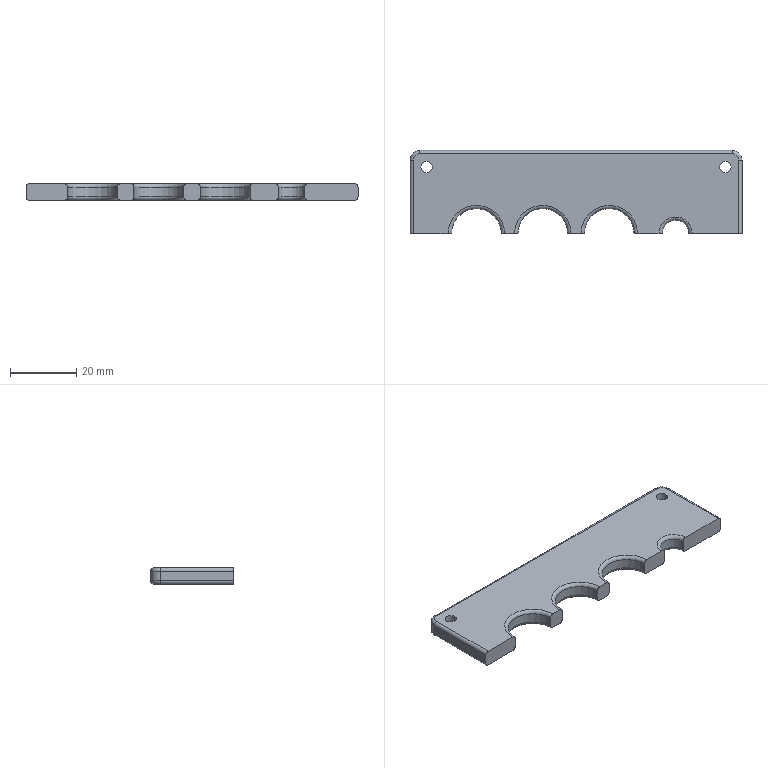Part | SolidWorks | features Fillet 2, Extrusion 1, HoleWzd 1, ICE 1 | 1 solid | 42 faces | box 100 x 25 x 5 mm | volume 10800 mm3 | cylinder 16 | torus 12 | plane 10 | cone 4 | commonest cylinder face diameters 2 x6 3.4 x4 15 x3 6 x2 8 x1
STEP:
#1=CARTESIAN_POINT('',(6.7,20.,1.66));
#2=VERTEX_POINT('',#1);
#3=CARTESIAN_POINT('',(3.3,20.,1.66));
#4=VERTEX_POINT('',#3);
#5=CARTESIAN_POINT('',(5.,20.,1.66));
#6=DIRECTION('',(0.,0.,-1.));
#7=DIRECTION('',(-1.,0.,0.));
#8=AXIS2_PLACEMENT_3D('',#5,#6,#7);
#9=CIRCLE('',#8,1.7);
#10=EDGE_CURVE('',#2,#4,#9,.T.);
#11=ORIENTED_EDGE('',*,*,#10,.F.);
#12=CARTESIAN_POINT('',(8.36,20.,0.));
#13=VERTEX_POINT('',#12);
#14=CARTESIAN_POINT('',(8.36,20.,0.));
#15=DIRECTION('',(0.7071,0.,-0.7071));
#16=VECTOR('',#15,1000.);
#17=LINE('',#14,#16);
#18=EDGE_CURVE('',#2,#13,#17,.T.);
#19=ORIENTED_EDGE('',*,*,#18,.T.);
#20=CARTESIAN_POINT('',(1.64,20.,0.));
#21=VERTEX_POINT('',#20);
#22=CARTESIAN_POINT('',(5.,20.,0.));
#23=DIRECTION('',(0.,0.,-1.));
#24=DIRECTION('',(-1.,0.,0.));
#25=AXIS2_PLACEMENT_3D('',#22,#23,#24);
#26=CIRCLE('',#25,3.36);
#27=EDGE_CURVE('',#13,#21,#26,.T.);
#28=ORIENTED_EDGE('',*,*,#27,.T.);
#29=CARTESIAN_POINT('',(1.64,20.,0.));
#30=DIRECTION('',(-0.7071,0.,-0.7071));
#31=VECTOR('',#30,1000.);
#32=LINE('',#29,#31);
#33=EDGE_CURVE('',#4,#21,#32,.T.);
#34=ORIENTED_EDGE('',*,*,#33,.F.);
#35=EDGE_LOOP('',(#11,#19,#28,#34));
#36=FACE_OUTER_BOUND('',#35,.T.);
#37=CARTESIAN_POINT('',(5.,20.,0.));
#38=DIRECTION('',(0.,0.,-1.));
#39=DIRECTION('',(-1.,0.,0.));
#40=AXIS2_PLACEMENT_3D('',#37,#38,#39);
#41=CONICAL_SURFACE('',#40,3.36,0.7854);
#42=ADVANCED_FACE('',(#36),#41,.F.);
#43=CARTESIAN_POINT('',(6.7,20.,5.));
#44=VERTEX_POINT('',#43);
#45=CARTESIAN_POINT('',(3.3,20.,5.));
#46=VERTEX_POINT('',#45);
#47=CARTESIAN_POINT('',(5.,20.,5.));
#48=DIRECTION('',(0.,0.,-1.));
#49=DIRECTION('',(-1.,0.,0.));
#50=AXIS2_PLACEMENT_3D('',#47,#48,#49);
#51=CIRCLE('',#50,1.7);
#52=EDGE_CURVE('',#44,#46,#51,.T.);
#53=ORIENTED_EDGE('',*,*,#52,.F.);
#54=CARTESIAN_POINT('',(6.7,20.,0.));
#55=DIRECTION('',(0.,0.,-1.));
#56=VECTOR('',#55,1000.);
#57=LINE('',#54,#56);
#58=EDGE_CURVE('',#44,#2,#57,.T.);
#59=ORIENTED_EDGE('',*,*,#58,.T.);
#60=ORIENTED_EDGE('',*,*,#10,.T.);
#61=CARTESIAN_POINT('',(3.3,20.,0.));
#62=DIRECTION('',(0.,0.,-1.));
#63=VECTOR('',#62,1000.);
#64=LINE('',#61,#63);
#65=EDGE_CURVE('',#46,#4,#64,.T.);
#66=ORIENTED_EDGE('',*,*,#65,.F.);
#67=EDGE_LOOP('',(#53,#59,#60,#66));
#68=FACE_OUTER_BOUND('',#67,.T.);
#69=CARTESIAN_POINT('',(5.,20.,0.));
#70=DIRECTION('',(0.,0.,-1.));
#71=DIRECTION('',(-1.,0.,0.));
#72=AXIS2_PLACEMENT_3D('',#69,#70,#71);
#73=CYLINDRICAL_SURFACE('',#72,1.7);
#74=ADVANCED_FACE('',(#68),#73,.F.);
#75=CARTESIAN_POINT('',(96.7,20.,1.66));
#76=VERTEX_POINT('',#75);
#77=CARTESIAN_POINT('',(93.3,20.,1.66));
#78=VERTEX_POINT('',#77);
#79=CARTESIAN_POINT('',(95.,20.,1.66));
#80=DIRECTION('',(0.,0.,-1.));
#81=DIRECTION('',(-1.,0.,0.));
#82=AXIS2_PLACEMENT_3D('',#79,#80,#81);
#83=CIRCLE('',#82,1.7);
#84=EDGE_CURVE('',#76,#78,#83,.T.);
#85=ORIENTED_EDGE('',*,*,#84,.F.);
#86=CARTESIAN_POINT('',(98.36,20.,0.));
#87=VERTEX_POINT('',#86);
#88=CARTESIAN_POINT('',(98.36,20.,0.));
#89=DIRECTION('',(0.7071,0.,-0.7071));
#90=VECTOR('',#89,1000.);
#91=LINE('',#88,#90);
#92=EDGE_CURVE('',#76,#87,#91,.T.);
#93=ORIENTED_EDGE('',*,*,#92,.T.);
#94=CARTESIAN_POINT('',(91.64,20.,0.));
#95=VERTEX_POINT('',#94);
#96=CARTESIAN_POINT('',(95.,20.,0.));
#97=DIRECTION('',(0.,0.,-1.));
#98=DIRECTION('',(-1.,0.,0.));
#99=AXIS2_PLACEMENT_3D('',#96,#97,#98);
#100=CIRCLE('',#99,3.36);
#101=EDGE_CURVE('',#87,#95,#100,.T.);
#102=ORIENTED_EDGE('',*,*,#101,.T.);
#103=CARTESIAN_POINT('',(91.64,20.,0.));
#104=DIRECTION('',(-0.7071,0.,-0.7071));
#105=VECTOR('',#104,1000.);
#106=LINE('',#103,#105);
#107=EDGE_CURVE('',#78,#95,#106,.T.);
#108=ORIENTED_EDGE('',*,*,#107,.F.);
#109=EDGE_LOOP('',(#85,#93,#102,#108));
#110=FACE_OUTER_BOUND('',#109,.T.);
#111=CARTESIAN_POINT('',(95.,20.,0.));
#112=DIRECTION('',(0.,0.,-1.));
#113=DIRECTION('',(-1.,0.,0.));
#114=AXIS2_PLACEMENT_3D('',#111,#112,#113);
#115=CONICAL_SURFACE('',#114,3.36,0.7854);
#116=ADVANCED_FACE('',(#110),#115,.F.);
#117=CARTESIAN_POINT('',(96.7,20.,5.));
#118=VERTEX_POINT('',#117);
#119=CARTESIAN_POINT('',(93.3,20.,5.));
#120=VERTEX_POINT('',#119);
#121=CARTESIAN_POINT('',(95.,20.,5.));
#122=DIRECTION('',(0.,0.,-1.));
#123=DIRECTION('',(-1.,0.,0.));
#124=AXIS2_PLACEMENT_3D('',#121,#122,#123);
#125=CIRCLE('',#124,1.7);
#126=EDGE_CURVE('',#118,#120,#125,.T.);
#127=ORIENTED_EDGE('',*,*,#126,.F.);
#128=CARTESIAN_POINT('',(96.7,20.,0.));
#129=DIRECTION('',(0.,0.,-1.));
#130=VECTOR('',#129,1000.);
#131=LINE('',#128,#130);
#132=EDGE_CURVE('',#118,#76,#131,.T.);
#133=ORIENTED_EDGE('',*,*,#132,.T.);
#134=ORIENTED_EDGE('',*,*,#84,.T.);
#135=CARTESIAN_POINT('',(93.3,20.,0.));
#136=DIRECTION('',(0.,0.,-1.));
#137=VECTOR('',#136,1000.);
#138=LINE('',#135,#137);
#139=EDGE_CURVE('',#120,#78,#138,.T.);
#140=ORIENTED_EDGE('',*,*,#139,.F.);
#141=EDGE_LOOP('',(#127,#133,#134,#140));
#142=FACE_OUTER_BOUND('',#141,.T.);
#143=CARTESIAN_POINT('',(95.,20.,0.));
#144=DIRECTION('',(0.,0.,-1.));
#145=DIRECTION('',(-1.,0.,0.));
#146=AXIS2_PLACEMENT_3D('',#143,#144,#145);
#147=CYLINDRICAL_SURFACE('',#146,1.7);
#148=ADVANCED_FACE('',(#142),#147,.F.);
#149=CARTESIAN_POINT('',(68.5,0.,5.));
#150=VERTEX_POINT('',#149);
#151=CARTESIAN_POINT('',(75.,0.,5.));
#152=VERTEX_POINT('',#151);
#153=CARTESIAN_POINT('',(0.,0.,5.));
#154=DIRECTION('',(1.,0.,0.));
#155=VECTOR('',#154,1000.);
#156=LINE('',#153,#155);
#157=EDGE_CURVE('',#150,#152,#156,.T.);
#158=ORIENTED_EDGE('',*,*,#157,.F.);
#159=CARTESIAN_POINT('',(67.5,0.,4.));
#160=VERTEX_POINT('',#159);
#161=CARTESIAN_POINT('',(68.5,0.,4.));
#162=DIRECTION('',(0.,-1.,0.));
#163=DIRECTION('',(0.,0.,1.));
#164=AXIS2_PLACEMENT_3D('',#161,#162,#163);
#165=CIRCLE('',#164,1.);
#166=EDGE_CURVE('',#150,#160,#165,.T.);
#167=ORIENTED_EDGE('',*,*,#166,.T.);
#168=CARTESIAN_POINT('',(67.5,0.,1.));
#169=VERTEX_POINT('',#168);
#170=CARTESIAN_POINT('',(67.5,0.,0.));
#171=DIRECTION('',(0.,0.,-1.));
#172=VECTOR('',#171,1000.);
#173=LINE('',#170,#172);
#174=EDGE_CURVE('',#160,#169,#173,.T.);
#175=ORIENTED_EDGE('',*,*,#174,.T.);
#176=CARTESIAN_POINT('',(68.5,0.,0.));
#177=VERTEX_POINT('',#176);
#178=CARTESIAN_POINT('',(68.5,0.,1.));
#179=DIRECTION('',(0.,-1.,0.));
#180=DIRECTION('',(0.,0.,1.));
#181=AXIS2_PLACEMENT_3D('',#178,#179,#180);
#182=CIRCLE('',#181,1.);
#183=EDGE_CURVE('',#169,#177,#182,.T.);
#184=ORIENTED_EDGE('',*,*,#183,.T.);
#185=CARTESIAN_POINT('',(75.,0.,0.));
#186=VERTEX_POINT('',#185);
#187=CARTESIAN_POINT('',(0.,0.,0.));
#188=DIRECTION('',(1.,0.,0.));
#189=VECTOR('',#188,1000.);
#190=LINE('',#187,#189);
#191=EDGE_CURVE('',#177,#186,#190,.T.);
#192=ORIENTED_EDGE('',*,*,#191,.T.);
#193=CARTESIAN_POINT('',(76.,0.,1.));
#194=VERTEX_POINT('',#193);
#195=CARTESIAN_POINT('',(75.,0.,1.));
#196=DIRECTION('',(0.,-1.,0.));
#197=DIRECTION('',(0.,0.,1.));
#198=AXIS2_PLACEMENT_3D('',#195,#196,#197);
#199=CIRCLE('',#198,1.);
#200=EDGE_CURVE('',#186,#194,#199,.T.);
#201=ORIENTED_EDGE('',*,*,#200,.T.);
#202=CARTESIAN_POINT('',(76.,0.,4.));
#203=VERTEX_POINT('',#202);
#204=CARTESIAN_POINT('',(76.,0.,0.));
#205=DIRECTION('',(0.,0.,1.));
#206=VECTOR('',#205,1000.);
#207=LINE('',#204,#206);
#208=EDGE_CURVE('',#194,#203,#207,.T.);
#209=ORIENTED_EDGE('',*,*,#208,.T.);
#210=CARTESIAN_POINT('',(75.,0.,4.));
#211=DIRECTION('',(0.,-1.,0.));
#212=DIRECTION('',(0.,0.,1.));
#213=AXIS2_PLACEMENT_3D('',#210,#211,#212);
#214=CIRCLE('',#213,1.);
#215=EDGE_CURVE('',#203,#152,#214,.T.);
#216=ORIENTED_EDGE('',*,*,#215,.T.);
#217=EDGE_LOOP('',(#158,#167,#175,#184,#192,#201,#209,#216));
#218=FACE_OUTER_BOUND('',#217,.T.);
#219=CARTESIAN_POINT('',(0.,0.,5.));
#220=DIRECTION('',(0.,1.,0.));
#221=DIRECTION('',(0.,0.,1.));
#222=AXIS2_PLACEMENT_3D('',#219,#220,#221);
#223=PLANE('',#222);
#224=ADVANCED_FACE('',(#218),#223,.F.);
#225=CARTESIAN_POINT('',(48.5,0.,5.));
#226=VERTEX_POINT('',#225);
#227=CARTESIAN_POINT('',(51.5,0.,5.));
#228=VERTEX_POINT('',#227);
#229=CARTESIAN_POINT('',(0.,0.,5.));
#230=DIRECTION('',(1.,0.,0.));
#231=VECTOR('',#230,1000.);
#232=LINE('',#229,#231);
#233=EDGE_CURVE('',#226,#228,#232,.T.);
#234=ORIENTED_EDGE('',*,*,#233,.F.);
#235=CARTESIAN_POINT('',(47.5,0.,4.));
#236=VERTEX_POINT('',#235);
#237=CARTESIAN_POINT('',(48.5,0.,4.));
#238=DIRECTION('',(0.,-1.,0.));
#239=DIRECTION('',(0.,0.,1.));
#240=AXIS2_PLACEMENT_3D('',#237,#238,#239);
#241=CIRCLE('',#240,1.);
#242=EDGE_CURVE('',#226,#236,#241,.T.);
#243=ORIENTED_EDGE('',*,*,#242,.T.);
#244=CARTESIAN_POINT('',(47.5,0.,1.));
#245=VERTEX_POINT('',#244);
#246=CARTESIAN_POINT('',(47.5,0.,0.));
#247=DIRECTION('',(0.,0.,-1.));
#248=VECTOR('',#247,1000.);
#249=LINE('',#246,#248);
#250=EDGE_CURVE('',#236,#245,#249,.T.);
#251=ORIENTED_EDGE('',*,*,#250,.T.);
#252=CARTESIAN_POINT('',(48.5,0.,0.));
#253=VERTEX_POINT('',#252);
#254=CARTESIAN_POINT('',(48.5,0.,1.));
#255=DIRECTION('',(0.,-1.,0.));
#256=DIRECTION('',(0.,0.,1.));
#257=AXIS2_PLACEMENT_3D('',#254,#255,#256);
#258=CIRCLE('',#257,1.);
#259=EDGE_CURVE('',#245,#253,#258,.T.);
#260=ORIENTED_EDGE('',*,*,#259,.T.);
#261=CARTESIAN_POINT('',(51.5,0.,0.));
#262=VERTEX_POINT('',#261);
#263=CARTESIAN_POINT('',(0.,0.,0.));
#264=DIRECTION('',(1.,0.,0.));
#265=VECTOR('',#264,1000.);
#266=LINE('',#263,#265);
#267=EDGE_CURVE('',#253,#262,#266,.T.);
#268=ORIENTED_EDGE('',*,*,#267,.T.);
#269=CARTESIAN_POINT('',(52.5,0.,1.));
#270=VERTEX_POINT('',#269);
#271=CARTESIAN_POINT('',(51.5,0.,1.));
#272=DIRECTION('',(0.,-1.,0.));
#273=DIRECTION('',(0.,0.,1.));
#274=AXIS2_PLACEMENT_3D('',#271,#272,#273);
#275=CIRCLE('',#274,1.);
#276=EDGE_CURVE('',#262,#270,#275,.T.);
#277=ORIENTED_EDGE('',*,*,#276,.T.);
#278=CARTESIAN_POINT('',(52.5,0.,4.));
#279=VERTEX_POINT('',#278);
#280=CARTESIAN_POINT('',(52.5,0.,0.));
#281=DIRECTION('',(0.,0.,1.));
#282=VECTOR('',#281,1000.);
#283=LINE('',#280,#282);
#284=EDGE_CURVE('',#270,#279,#283,.T.);
#285=ORIENTED_EDGE('',*,*,#284,.T.);
#286=CARTESIAN_POINT('',(51.5,0.,4.));
#287=DIRECTION('',(0.,-1.,0.));
#288=DIRECTION('',(0.,0.,1.));
#289=AXIS2_PLACEMENT_3D('',#286,#287,#288);
#290=CIRCLE('',#289,1.);
#291=EDGE_CURVE('',#279,#228,#290,.T.);
#292=ORIENTED_EDGE('',*,*,#291,.T.);
#293=EDGE_LOOP('',(#234,#243,#251,#260,#268,#277,#285,#292));
#294=FACE_OUTER_BOUND('',#293,.T.);
#295=CARTESIAN_POINT('',(0.,0.,5.));
#296=DIRECTION('',(0.,1.,0.));
#297=DIRECTION('',(0.,0.,1.));
#298=AXIS2_PLACEMENT_3D('',#295,#296,#297);
#299=PLANE('',#298);
#300=ADVANCED_FACE('',(#294),#299,.F.);
#301=CARTESIAN_POINT('',(28.5,0.,5.));
#302=VERTEX_POINT('',#301);
#303=CARTESIAN_POINT('',(31.5,0.,5.));
#304=VERTEX_POINT('',#303);
#305=CARTESIAN_POINT('',(0.,0.,5.));
#306=DIRECTION('',(1.,0.,0.));
#307=VECTOR('',#306,1000.);
#308=LINE('',#305,#307);
#309=EDGE_CURVE('',#302,#304,#308,.T.);
#310=ORIENTED_EDGE('',*,*,#309,.F.);
#311=CARTESIAN_POINT('',(27.5,0.,4.));
#312=VERTEX_POINT('',#311);
#313=CARTESIAN_POINT('',(28.5,0.,4.));
#314=DIRECTION('',(0.,-1.,0.));
#315=DIRECTION('',(0.,0.,1.));
#316=AXIS2_PLACEMENT_3D('',#313,#314,#315);
#317=CIRCLE('',#316,1.);
#318=EDGE_CURVE('',#302,#312,#317,.T.);
#319=ORIENTED_EDGE('',*,*,#318,.T.);
#320=CARTESIAN_POINT('',(27.5,0.,1.));
#321=VERTEX_POINT('',#320);
#322=CARTESIAN_POINT('',(27.5,0.,0.));
#323=DIRECTION('',(0.,0.,-1.));
#324=VECTOR('',#323,1000.);
#325=LINE('',#322,#324);
#326=EDGE_CURVE('',#312,#321,#325,.T.);
#327=ORIENTED_EDGE('',*,*,#326,.T.);
#328=CARTESIAN_POINT('',(28.5,0.,0.));
#329=VERTEX_POINT('',#328);
#330=CARTESIAN_POINT('',(28.5,0.,1.));
#331=DIRECTION('',(0.,-1.,0.));
#332=DIRECTION('',(0.,0.,1.));
#333=AXIS2_PLACEMENT_3D('',#330,#331,#332);
#334=CIRCLE('',#333,1.);
#335=EDGE_CURVE('',#321,#329,#334,.T.);
#336=ORIENTED_EDGE('',*,*,#335,.T.);
#337=CARTESIAN_POINT('',(31.5,0.,0.));
#338=VERTEX_POINT('',#337);
#339=CARTESIAN_POINT('',(0.,0.,0.));
#340=DIRECTION('',(1.,0.,0.));
#341=VECTOR('',#340,1000.);
#342=LINE('',#339,#341);
#343=EDGE_CURVE('',#329,#338,#342,.T.);
#344=ORIENTED_EDGE('',*,*,#343,.T.);
#345=CARTESIAN_POINT('',(32.5,0.,1.));
#346=VERTEX_POINT('',#345);
#347=CARTESIAN_POINT('',(31.5,0.,1.));
#348=DIRECTION('',(0.,-1.,0.));
#349=DIRECTION('',(0.,0.,1.));
#350=AXIS2_PLACEMENT_3D('',#347,#348,#349);
#351=CIRCLE('',#350,1.);
#352=EDGE_CURVE('',#338,#346,#351,.T.);
#353=ORIENTED_EDGE('',*,*,#352,.T.);
#354=CARTESIAN_POINT('',(32.5,0.,4.));
#355=VERTEX_POINT('',#354);
#356=CARTESIAN_POINT('',(32.5,0.,0.));
#357=DIRECTION('',(0.,0.,1.));
#358=VECTOR('',#357,1000.);
#359=LINE('',#356,#358);
#360=EDGE_CURVE('',#346,#355,#359,.T.);
#361=ORIENTED_EDGE('',*,*,#360,.T.);
#362=CARTESIAN_POINT('',(31.5,0.,4.));
#363=DIRECTION('',(0.,-1.,0.));
#364=DIRECTION('',(0.,0.,1.));
#365=AXIS2_PLACEMENT_3D('',#362,#363,#364);
#366=CIRCLE('',#365,1.);
#367=EDGE_CURVE('',#355,#304,#366,.T.);
#368=ORIENTED_EDGE('',*,*,#367,.T.);
#369=EDGE_LOOP('',(#310,#319,#327,#336,#344,#353,#361,#368));
#370=FACE_OUTER_BOUND('',#369,.T.);
#371=CARTESIAN_POINT('',(0.,0.,5.));
#372=DIRECTION('',(0.,1.,0.));
#373=DIRECTION('',(0.,0.,1.));
#374=AXIS2_PLACEMENT_3D('',#371,#372,#373);
#375=PLANE('',#374);
#376=ADVANCED_FACE('',(#370),#375,.F.);
#377=CARTESIAN_POINT('',(12.5,0.,1.));
#378=VERTEX_POINT('',#377);
#379=CARTESIAN_POINT('',(12.5,0.,4.));
#380=VERTEX_POINT('',#379);
#381=CARTESIAN_POINT('',(12.5,0.,0.));
#382=DIRECTION('',(0.,0.,1.));
#383=VECTOR('',#382,1000.);
#384=LINE('',#381,#383);
#385=EDGE_CURVE('',#378,#380,#384,.T.);
#386=ORIENTED_EDGE('',*,*,#385,.T.);
#387=CARTESIAN_POINT('',(11.5,0.,5.));
#388=VERTEX_POINT('',#387);
#389=CARTESIAN_POINT('',(11.5,0.,4.));
#390=DIRECTION('',(0.,-1.,0.));
#391=DIRECTION('',(0.,0.,1.));
#392=AXIS2_PLACEMENT_3D('',#389,#390,#391);
#393=CIRCLE('',#392,1.);
#394=EDGE_CURVE('',#380,#388,#393,.T.);
#395=ORIENTED_EDGE('',*,*,#394,.T.);
#396=CARTESIAN_POINT('',(1.,0.,5.));
#397=VERTEX_POINT('',#396);
#398=CARTESIAN_POINT('',(0.,0.,5.));
#399=DIRECTION('',(1.,0.,0.));
#400=VECTOR('',#399,1000.);
#401=LINE('',#398,#400);
#402=EDGE_CURVE('',#397,#388,#401,.T.);
#403=ORIENTED_EDGE('',*,*,#402,.F.);
#404=CARTESIAN_POINT('',(0.,0.,4.));
#405=VERTEX_POINT('',#404);
#406=CARTESIAN_POINT('',(1.,0.,4.));
#407=DIRECTION('',(0.,-1.,0.));
#408=DIRECTION('',(0.,0.,1.));
#409=AXIS2_PLACEMENT_3D('',#406,#407,#408);
#410=CIRCLE('',#409,1.);
#411=EDGE_CURVE('',#397,#405,#410,.T.);
#412=ORIENTED_EDGE('',*,*,#411,.T.);
#413=CARTESIAN_POINT('',(0.,0.,1.));
#414=VERTEX_POINT('',#413);
#415=CARTESIAN_POINT('',(0.,0.,5.));
#416=DIRECTION('',(0.,0.,-1.));
#417=VECTOR('',#416,1000.);
#418=LINE('',#415,#417);
#419=EDGE_CURVE('',#405,#414,#418,.T.);
#420=ORIENTED_EDGE('',*,*,#419,.T.);
#421=CARTESIAN_POINT('',(1.,0.,0.));
#422=VERTEX_POINT('',#421);
#423=CARTESIAN_POINT('',(1.,0.,1.));
#424=DIRECTION('',(0.,-1.,0.));
#425=DIRECTION('',(0.,0.,1.));
#426=AXIS2_PLACEMENT_3D('',#423,#424,#425);
#427=CIRCLE('',#426,1.);
#428=EDGE_CURVE('',#414,#422,#427,.T.);
#429=ORIENTED_EDGE('',*,*,#428,.T.);
#430=CARTESIAN_POINT('',(11.5,0.,0.));
#431=VERTEX_POINT('',#430);
#432=CARTESIAN_POINT('',(0.,0.,0.));
#433=DIRECTION('',(1.,0.,0.));
#434=VECTOR('',#433,1000.);
#435=LINE('',#432,#434);
#436=EDGE_CURVE('',#422,#431,#435,.T.);
#437=ORIENTED_EDGE('',*,*,#436,.T.);
#438=CARTESIAN_POINT('',(11.5,0.,1.));
#439=DIRECTION('',(0.,-1.,0.));
#440=DIRECTION('',(0.,0.,1.));
#441=AXIS2_PLACEMENT_3D('',#438,#439,#440);
#442=CIRCLE('',#441,1.);
#443=EDGE_CURVE('',#431,#378,#442,.T.);
#444=ORIENTED_EDGE('',*,*,#443,.T.);
#445=EDGE_LOOP('',(#386,#395,#403,#412,#420,#429,#437,#444));
#446=FACE_OUTER_BOUND('',#445,.T.);
#447=CARTESIAN_POINT('',(0.,0.,5.));
#448=DIRECTION('',(0.,1.,0.));
#449=DIRECTION('',(0.,0.,1.));
#450=AXIS2_PLACEMENT_3D('',#447,#448,#449);
#451=PLANE('',#450);
#452=ADVANCED_FACE('',(#446),#451,.F.);
#453=ORIENTED_EDGE('',*,*,#419,.F.);
#454=CARTESIAN_POINT('',(0.,22.,4.));
#455=VERTEX_POINT('',#454);
#456=CARTESIAN_POINT('',(0.,0.,4.));
#457=DIRECTION('',(0.,1.,0.));
#458=VECTOR('',#457,1000.);
#459=LINE('',#456,#458);
#460=EDGE_CURVE('',#405,#455,#459,.T.);
#461=ORIENTED_EDGE('',*,*,#460,.T.);
#462=CARTESIAN_POINT('',(0.,22.,1.));
#463=VERTEX_POINT('',#462);
#464=CARTESIAN_POINT('',(0.,22.,5.));
#465=DIRECTION('',(0.,0.,-1.));
#466=VECTOR('',#465,1000.);
#467=LINE('',#464,#466);
#468=EDGE_CURVE('',#455,#463,#467,.T.);
#469=ORIENTED_EDGE('',*,*,#468,.T.);
#470=CARTESIAN_POINT('',(0.,0.,1.));
#471=DIRECTION('',(0.,-1.,0.));
#472=VECTOR('',#471,1000.);
#473=LINE('',#470,#472);
#474=EDGE_CURVE('',#463,#414,#473,.T.);
#475=ORIENTED_EDGE('',*,*,#474,.T.);
#476=EDGE_LOOP('',(#453,#461,#469,#475));
#477=FACE_OUTER_BOUND('',#476,.T.);
#478=CARTESIAN_POINT('',(0.,0.,5.));
#479=DIRECTION('',(1.,0.,0.));
#480=DIRECTION('',(0.,0.,-1.));
#481=AXIS2_PLACEMENT_3D('',#478,#479,#480);
#482=PLANE('',#481);
#483=ADVANCED_FACE('',(#477),#482,.F.);
#484=CARTESIAN_POINT('',(85.,0.,5.));
#485=VERTEX_POINT('',#484);
#486=CARTESIAN_POINT('',(99.,0.,5.));
#487=VERTEX_POINT('',#486);
#488=CARTESIAN_POINT('',(0.,0.,5.));
#489=DIRECTION('',(1.,0.,0.));
#490=VECTOR('',#489,1000.);
#491=LINE('',#488,#490);
#492=EDGE_CURVE('',#485,#487,#491,.T.);
#493=ORIENTED_EDGE('',*,*,#492,.F.);
#494=CARTESIAN_POINT('',(84.,0.,4.));
#495=VERTEX_POINT('',#494);
#496=CARTESIAN_POINT('',(85.,0.,4.));
#497=DIRECTION('',(0.,-1.,0.));
#498=DIRECTION('',(0.,0.,1.));
#499=AXIS2_PLACEMENT_3D('',#496,#497,#498);
#500=CIRCLE('',#499,1.);
#501=EDGE_CURVE('',#485,#495,#500,.T.);
#502=ORIENTED_EDGE('',*,*,#501,.T.);
#503=CARTESIAN_POINT('',(84.,0.,1.));
#504=VERTEX_POINT('',#503);
#505=CARTESIAN_POINT('',(84.,0.,0.));
#506=DIRECTION('',(0.,0.,-1.));
#507=VECTOR('',#506,1000.);
#508=LINE('',#505,#507);
#509=EDGE_CURVE('',#495,#504,#508,.T.);
#510=ORIENTED_EDGE('',*,*,#509,.T.);
#511=CARTESIAN_POINT('',(85.,0.,0.));
#512=VERTEX_POINT('',#511);
#513=CARTESIAN_POINT('',(85.,0.,1.));
#514=DIRECTION('',(0.,-1.,0.));
#515=DIRECTION('',(0.,0.,1.));
#516=AXIS2_PLACEMENT_3D('',#513,#514,#515);
#517=CIRCLE('',#516,1.);
#518=EDGE_CURVE('',#504,#512,#517,.T.);
#519=ORIENTED_EDGE('',*,*,#518,.T.);
#520=CARTESIAN_POINT('',(99.,0.,0.));
#521=VERTEX_POINT('',#520);
#522=CARTESIAN_POINT('',(0.,0.,0.));
#523=DIRECTION('',(1.,0.,0.));
#524=VECTOR('',#523,1000.);
#525=LINE('',#522,#524);
#526=EDGE_CURVE('',#512,#521,#525,.T.);
#527=ORIENTED_EDGE('',*,*,#526,.T.);
#528=CARTESIAN_POINT('',(100.,0.,1.));
#529=VERTEX_POINT('',#528);
#530=CARTESIAN_POINT('',(99.,0.,1.));
#531=DIRECTION('',(0.,-1.,0.));
#532=DIRECTION('',(0.,0.,1.));
#533=AXIS2_PLACEMENT_3D('',#530,#531,#532);
#534=CIRCLE('',#533,1.);
#535=EDGE_CURVE('',#521,#529,#534,.T.);
#536=ORIENTED_EDGE('',*,*,#535,.T.);
#537=CARTESIAN_POINT('',(100.,0.,4.));
#538=VERTEX_POINT('',#537);
#539=CARTESIAN_POINT('',(100.,0.,5.));
#540=DIRECTION('',(0.,0.,-1.));
#541=VECTOR('',#540,1000.);
#542=LINE('',#539,#541);
#543=EDGE_CURVE('',#538,#529,#542,.T.);
#544=ORIENTED_EDGE('',*,*,#543,.F.);
#545=CARTESIAN_POINT('',(99.,0.,4.));
#546=DIRECTION('',(0.,-1.,0.));
#547=DIRECTION('',(0.,0.,1.));
#548=AXIS2_PLACEMENT_3D('',#545,#546,#547);
#549=CIRCLE('',#548,1.);
#550=EDGE_CURVE('',#538,#487,#549,.T.);
#551=ORIENTED_EDGE('',*,*,#550,.T.);
#552=EDGE_LOOP('',(#493,#502,#510,#519,#527,#536,#544,#551));
#553=FACE_OUTER_BOUND('',#552,.T.);
#554=CARTESIAN_POINT('',(0.,0.,5.));
#555=DIRECTION('',(0.,1.,0.));
#556=DIRECTION('',(0.,0.,1.));
#557=AXIS2_PLACEMENT_3D('',#554,#555,#556);
#558=PLANE('',#557);
#559=ADVANCED_FACE('',(#553),#558,.F.);
#560=CARTESIAN_POINT('',(100.,22.,1.));
#561=VERTEX_POINT('',#560);
#562=CARTESIAN_POINT('',(100.,22.,4.));
#563=VERTEX_POINT('',#562);
#564=CARTESIAN_POINT('',(100.,22.,5.));
#565=DIRECTION('',(0.,0.,1.));
#566=VECTOR('',#565,1000.);
#567=LINE('',#564,#566);
#568=EDGE_CURVE('',#561,#563,#567,.T.);
#569=ORIENTED_EDGE('',*,*,#568,.T.);
#570=CARTESIAN_POINT('',(100.,0.,4.));
#571=DIRECTION('',(0.,-1.,0.));
#572=VECTOR('',#571,1000.);
#573=LINE('',#570,#572);
#574=EDGE_CURVE('',#563,#538,#573,.T.);
#575=ORIENTED_EDGE('',*,*,#574,.T.);
#576=ORIENTED_EDGE('',*,*,#543,.T.);
#577=CARTESIAN_POINT('',(100.,22.,1.));
#578=DIRECTION('',(0.,1.,0.));
#579=VECTOR('',#578,1000.);
#580=LINE('',#577,#579);
#581=EDGE_CURVE('',#529,#561,#580,.T.);
#582=ORIENTED_EDGE('',*,*,#581,.T.);
#583=EDGE_LOOP('',(#569,#575,#576,#582));
#584=FACE_OUTER_BOUND('',#583,.T.);
#585=CARTESIAN_POINT('',(100.,0.,5.));
#586=DIRECTION('',(-1.,0.,0.));
#587=DIRECTION('',(0.,0.,1.));
#588=AXIS2_PLACEMENT_3D('',#585,#586,#587);
#589=PLANE('',#588);
#590=ADVANCED_FACE('',(#584),#589,.F.);
#591=CARTESIAN_POINT('',(3.,25.,1.));
#592=VERTEX_POINT('',#591);
#593=CARTESIAN_POINT('',(3.,25.,4.));
#594=VERTEX_POINT('',#593);
#595=CARTESIAN_POINT('',(3.,25.,5.));
#596=DIRECTION('',(0.,0.,1.));
#597=VECTOR('',#596,1000.);
#598=LINE('',#595,#597);
#599=EDGE_CURVE('',#592,#594,#598,.T.);
#600=ORIENTED_EDGE('',*,*,#599,.T.);
#601=CARTESIAN_POINT('',(97.,25.,4.));
#602=VERTEX_POINT('',#601);
#603=CARTESIAN_POINT('',(0.,25.,4.));
#604=DIRECTION('',(1.,0.,0.));
#605=VECTOR('',#604,1000.);
#606=LINE('',#603,#605);
#607=EDGE_CURVE('',#594,#602,#606,.T.);
#608=ORIENTED_EDGE('',*,*,#607,.T.);
#609=CARTESIAN_POINT('',(97.,25.,1.));
#610=VERTEX_POINT('',#609);
#611=CARTESIAN_POINT('',(97.,25.,5.));
#612=DIRECTION('',(0.,0.,-1.));
#613=VECTOR('',#612,1000.);
#614=LINE('',#611,#613);
#615=EDGE_CURVE('',#602,#610,#614,.T.);
#616=ORIENTED_EDGE('',*,*,#615,.T.);
#617=CARTESIAN_POINT('',(3.,25.,1.));
#618=DIRECTION('',(-1.,0.,0.));
#619=VECTOR('',#618,1000.);
#620=LINE('',#617,#619);
#621=EDGE_CURVE('',#610,#592,#620,.T.);
#622=ORIENTED_EDGE('',*,*,#621,.T.);
#623=EDGE_LOOP('',(#600,#608,#616,#622));
#624=FACE_OUTER_BOUND('',#623,.T.);
#625=CARTESIAN_POINT('',(0.,25.,5.));
#626=DIRECTION('',(0.,-1.,0.));
#627=DIRECTION('',(0.,0.,-1.));
#628=AXIS2_PLACEMENT_3D('',#625,#626,#627);
#629=PLANE('',#628);
#630=ADVANCED_FACE('',(#624),#629,.F.);
#631=CARTESIAN_POINT('',(5.,20.,5.));
#632=DIRECTION('',(0.,0.,-1.));
#633=DIRECTION('',(-1.,0.,0.));
#634=AXIS2_PLACEMENT_3D('',#631,#632,#633);
#635=CIRCLE('',#634,1.7);
#636=EDGE_CURVE('',#46,#44,#635,.T.);
#637=ORIENTED_EDGE('',*,*,#636,.T.);
#638=ORIENTED_EDGE('',*,*,#52,.T.);
#639=EDGE_LOOP('',(#637,#638));
#640=FACE_BOUND('',#639,.T.);
#641=CARTESIAN_POINT('',(95.,20.,5.));
#642=DIRECTION('',(0.,0.,-1.));
#643=DIRECTION('',(-1.,0.,0.));
#644=AXIS2_PLACEMENT_3D('',#641,#642,#643);
#645=CIRCLE('',#644,1.7);
#646=EDGE_CURVE('',#120,#118,#645,.T.);
#647=ORIENTED_EDGE('',*,*,#646,.T.);
#648=ORIENTED_EDGE('',*,*,#126,.T.);
#649=EDGE_LOOP('',(#647,#648));
#650=FACE_BOUND('',#649,.T.);
#651=ORIENTED_EDGE('',*,*,#402,.T.);
#652=CARTESIAN_POINT('',(20.,0.,5.));
#653=DIRECTION('',(0.,0.,-1.));
#654=DIRECTION('',(-1.,0.,0.));
#655=AXIS2_PLACEMENT_3D('',#652,#653,#654);
#656=CIRCLE('',#655,8.5);
#657=EDGE_CURVE('',#388,#302,#656,.T.);
#658=ORIENTED_EDGE('',*,*,#657,.T.);
#659=ORIENTED_EDGE('',*,*,#309,.T.);
#660=CARTESIAN_POINT('',(40.,0.,5.));
#661=DIRECTION('',(0.,0.,-1.));
#662=DIRECTION('',(-1.,0.,0.));
#663=AXIS2_PLACEMENT_3D('',#660,#661,#662);
#664=CIRCLE('',#663,8.5);
#665=EDGE_CURVE('',#304,#226,#664,.T.);
#666=ORIENTED_EDGE('',*,*,#665,.T.);
#667=ORIENTED_EDGE('',*,*,#233,.T.);
#668=CARTESIAN_POINT('',(60.,0.,5.));
#669=DIRECTION('',(0.,0.,-1.));
#670=DIRECTION('',(-1.,0.,0.));
#671=AXIS2_PLACEMENT_3D('',#668,#669,#670);
#672=CIRCLE('',#671,8.5);
#673=EDGE_CURVE('',#228,#150,#672,.T.);
#674=ORIENTED_EDGE('',*,*,#673,.T.);
#675=ORIENTED_EDGE('',*,*,#157,.T.);
#676=CARTESIAN_POINT('',(80.,0.,5.));
#677=DIRECTION('',(0.,0.,-1.));
#678=DIRECTION('',(-1.,0.,0.));
#679=AXIS2_PLACEMENT_3D('',#676,#677,#678);
#680=CIRCLE('',#679,5.);
#681=EDGE_CURVE('',#152,#485,#680,.T.);
#682=ORIENTED_EDGE('',*,*,#681,.T.);
#683=ORIENTED_EDGE('',*,*,#492,.T.);
#684=CARTESIAN_POINT('',(99.,22.,5.));
#685=VERTEX_POINT('',#684);
#686=CARTESIAN_POINT('',(99.,0.,5.));
#687=DIRECTION('',(0.,1.,0.));
#688=VECTOR('',#687,1000.);
#689=LINE('',#686,#688);
#690=EDGE_CURVE('',#487,#685,#689,.T.);
#691=ORIENTED_EDGE('',*,*,#690,.T.);
#692=CARTESIAN_POINT('',(97.,24.,5.));
#693=VERTEX_POINT('',#692);
#694=CARTESIAN_POINT('',(97.,22.,5.));
#695=DIRECTION('',(0.,0.,1.));
#696=DIRECTION('',(-1.,0.,0.));
#697=AXIS2_PLACEMENT_3D('',#694,#695,#696);
#698=CIRCLE('',#697,2.);
#699=EDGE_CURVE('',#685,#693,#698,.T.);
#700=ORIENTED_EDGE('',*,*,#699,.T.);
#701=CARTESIAN_POINT('',(3.,24.,5.));
#702=VERTEX_POINT('',#701);
#703=CARTESIAN_POINT('',(0.,24.,5.));
#704=DIRECTION('',(-1.,0.,0.));
#705=VECTOR('',#704,1000.);
#706=LINE('',#703,#705);
#707=EDGE_CURVE('',#693,#702,#706,.T.);
#708=ORIENTED_EDGE('',*,*,#707,.T.);
#709=CARTESIAN_POINT('',(1.,22.,5.));
#710=VERTEX_POINT('',#709);
#711=CARTESIAN_POINT('',(3.,22.,5.));
#712=DIRECTION('',(0.,0.,1.));
#713=DIRECTION('',(-1.,0.,0.));
#714=AXIS2_PLACEMENT_3D('',#711,#712,#713);
#715=CIRCLE('',#714,2.);
#716=EDGE_CURVE('',#702,#710,#715,.T.);
#717=ORIENTED_EDGE('',*,*,#716,.T.);
#718=CARTESIAN_POINT('',(1.,0.,5.));
#719=DIRECTION('',(0.,-1.,0.));
#720=VECTOR('',#719,1000.);
#721=LINE('',#718,#720);
#722=EDGE_CURVE('',#710,#397,#721,.T.);
#723=ORIENTED_EDGE('',*,*,#722,.T.);
#724=EDGE_LOOP('',(#651,#658,#659,#666,#667,#674,#675,#682,#683,#691,#700,#708,#717,#723));
#725=FACE_OUTER_BOUND('',#724,.T.);
#726=CARTESIAN_POINT('',(0.,0.,5.));
#727=DIRECTION('',(0.,0.,-1.));
#728=DIRECTION('',(-1.,0.,0.));
#729=AXIS2_PLACEMENT_3D('',#726,#727,#728);
#730=PLANE('',#729);
#731=ADVANCED_FACE('',(#640,#650,#725),#730,.F.);
#732=CARTESIAN_POINT('',(5.,20.,0.));
#733=DIRECTION('',(0.,0.,-1.));
#734=DIRECTION('',(-1.,0.,0.));
#735=AXIS2_PLACEMENT_3D('',#732,#733,#734);
#736=CIRCLE('',#735,3.36);
#737=EDGE_CURVE('',#21,#13,#736,.T.);
#738=ORIENTED_EDGE('',*,*,#737,.F.);
#739=ORIENTED_EDGE('',*,*,#27,.F.);
#740=EDGE_LOOP('',(#738,#739));
#741=FACE_BOUND('',#740,.T.);
#742=CARTESIAN_POINT('',(95.,20.,0.));
#743=DIRECTION('',(0.,0.,-1.));
#744=DIRECTION('',(-1.,0.,0.));
#745=AXIS2_PLACEMENT_3D('',#742,#743,#744);
#746=CIRCLE('',#745,3.36);
#747=EDGE_CURVE('',#95,#87,#746,.T.);
#748=ORIENTED_EDGE('',*,*,#747,.F.);
#749=ORIENTED_EDGE('',*,*,#101,.F.);
#750=EDGE_LOOP('',(#748,#749));
#751=FACE_BOUND('',#750,.T.);
#752=ORIENTED_EDGE('',*,*,#436,.F.);
#753=CARTESIAN_POINT('',(1.,22.,0.));
#754=VERTEX_POINT('',#753);
#755=CARTESIAN_POINT('',(1.,22.,0.));
#756=DIRECTION('',(0.,1.,0.));
#757=VECTOR('',#756,1000.);
#758=LINE('',#755,#757);
#759=EDGE_CURVE('',#422,#754,#758,.T.);
#760=ORIENTED_EDGE('',*,*,#759,.T.);
#761=CARTESIAN_POINT('',(3.,24.,0.));
#762=VERTEX_POINT('',#761);
#763=CARTESIAN_POINT('',(3.,22.,0.));
#764=DIRECTION('',(0.,0.,-1.));
#765=DIRECTION('',(-1.,0.,0.));
#766=AXIS2_PLACEMENT_3D('',#763,#764,#765);
#767=CIRCLE('',#766,2.);
#768=EDGE_CURVE('',#754,#762,#767,.T.);
#769=ORIENTED_EDGE('',*,*,#768,.T.);
#770=CARTESIAN_POINT('',(97.,24.,0.));
#771=VERTEX_POINT('',#770);
#772=CARTESIAN_POINT('',(97.,24.,0.));
#773=DIRECTION('',(1.,0.,0.));
#774=VECTOR('',#773,1000.);
#775=LINE('',#772,#774);
#776=EDGE_CURVE('',#762,#771,#775,.T.);
#777=ORIENTED_EDGE('',*,*,#776,.T.);
#778=CARTESIAN_POINT('',(99.,22.,0.));
#779=VERTEX_POINT('',#778);
#780=CARTESIAN_POINT('',(97.,22.,0.));
#781=DIRECTION('',(0.,0.,-1.));
#782=DIRECTION('',(-1.,0.,0.));
#783=AXIS2_PLACEMENT_3D('',#780,#781,#782);
#784=CIRCLE('',#783,2.);
#785=EDGE_CURVE('',#771,#779,#784,.T.);
#786=ORIENTED_EDGE('',*,*,#785,.T.);
#787=CARTESIAN_POINT('',(99.,0.,0.));
#788=DIRECTION('',(0.,-1.,0.));
#789=VECTOR('',#788,1000.);
#790=LINE('',#787,#789);
#791=EDGE_CURVE('',#779,#521,#790,.T.);
#792=ORIENTED_EDGE('',*,*,#791,.T.);
#793=ORIENTED_EDGE('',*,*,#526,.F.);
#794=CARTESIAN_POINT('',(80.,0.,0.));
#795=DIRECTION('',(0.,0.,1.));
#796=DIRECTION('',(-1.,0.,0.));
#797=AXIS2_PLACEMENT_3D('',#794,#795,#796);
#798=CIRCLE('',#797,5.);
#799=EDGE_CURVE('',#512,#186,#798,.T.);
#800=ORIENTED_EDGE('',*,*,#799,.T.);
#801=ORIENTED_EDGE('',*,*,#191,.F.);
#802=CARTESIAN_POINT('',(60.,0.,0.));
#803=DIRECTION('',(0.,0.,1.));
#804=DIRECTION('',(-1.,0.,0.));
#805=AXIS2_PLACEMENT_3D('',#802,#803,#804);
#806=CIRCLE('',#805,8.5);
#807=EDGE_CURVE('',#177,#262,#806,.T.);
#808=ORIENTED_EDGE('',*,*,#807,.T.);
#809=ORIENTED_EDGE('',*,*,#267,.F.);
#810=CARTESIAN_POINT('',(40.,0.,0.));
#811=DIRECTION('',(0.,0.,1.));
#812=DIRECTION('',(-1.,0.,0.));
#813=AXIS2_PLACEMENT_3D('',#810,#811,#812);
#814=CIRCLE('',#813,8.5);
#815=EDGE_CURVE('',#253,#338,#814,.T.);
#816=ORIENTED_EDGE('',*,*,#815,.T.);
#817=ORIENTED_EDGE('',*,*,#343,.F.);
#818=CARTESIAN_POINT('',(20.,0.,0.));
#819=DIRECTION('',(0.,0.,1.));
#820=DIRECTION('',(-1.,0.,0.));
#821=AXIS2_PLACEMENT_3D('',#818,#819,#820);
#822=CIRCLE('',#821,8.5);
#823=EDGE_CURVE('',#329,#431,#822,.T.);
#824=ORIENTED_EDGE('',*,*,#823,.T.);
#825=EDGE_LOOP('',(#752,#760,#769,#777,#786,#792,#793,#800,#801,#808,#809,#816,#817,#824));
#826=FACE_OUTER_BOUND('',#825,.T.);
#827=CARTESIAN_POINT('',(0.,0.,0.));
#828=DIRECTION('',(0.,0.,-1.));
#829=DIRECTION('',(-1.,0.,0.));
#830=AXIS2_PLACEMENT_3D('',#827,#828,#829);
#831=PLANE('',#830);
#832=ADVANCED_FACE('',(#741,#751,#826),#831,.T.);
#833=ORIENTED_EDGE('',*,*,#326,.F.);
#834=CARTESIAN_POINT('',(20.,0.,4.));
#835=DIRECTION('',(0.,0.,1.));
#836=DIRECTION('',(-1.,0.,0.));
#837=AXIS2_PLACEMENT_3D('',#834,#835,#836);
#838=CIRCLE('',#837,7.5);
#839=EDGE_CURVE('',#312,#380,#838,.T.);
#840=ORIENTED_EDGE('',*,*,#839,.T.);
#841=ORIENTED_EDGE('',*,*,#385,.F.);
#842=CARTESIAN_POINT('',(20.,0.,1.));
#843=DIRECTION('',(0.,0.,-1.));
#844=DIRECTION('',(-1.,0.,0.));
#845=AXIS2_PLACEMENT_3D('',#842,#843,#844);
#846=CIRCLE('',#845,7.5);
#847=EDGE_CURVE('',#378,#321,#846,.T.);
#848=ORIENTED_EDGE('',*,*,#847,.T.);
#849=EDGE_LOOP('',(#833,#840,#841,#848));
#850=FACE_OUTER_BOUND('',#849,.T.);
#851=CARTESIAN_POINT('',(20.,0.,0.));
#852=DIRECTION('',(0.,0.,1.));
#853=DIRECTION('',(1.,0.,0.));
#854=AXIS2_PLACEMENT_3D('',#851,#852,#853);
#855=CYLINDRICAL_SURFACE('',#854,7.5);
#856=ADVANCED_FACE('',(#850),#855,.F.);
#857=ORIENTED_EDGE('',*,*,#250,.F.);
#858=CARTESIAN_POINT('',(40.,0.,4.));
#859=DIRECTION('',(0.,0.,1.));
#860=DIRECTION('',(-1.,0.,0.));
#861=AXIS2_PLACEMENT_3D('',#858,#859,#860);
#862=CIRCLE('',#861,7.5);
#863=EDGE_CURVE('',#236,#355,#862,.T.);
#864=ORIENTED_EDGE('',*,*,#863,.T.);
#865=ORIENTED_EDGE('',*,*,#360,.F.);
#866=CARTESIAN_POINT('',(40.,0.,1.));
#867=DIRECTION('',(0.,0.,-1.));
#868=DIRECTION('',(-1.,0.,0.));
#869=AXIS2_PLACEMENT_3D('',#866,#867,#868);
#870=CIRCLE('',#869,7.5);
#871=EDGE_CURVE('',#346,#245,#870,.T.);
#872=ORIENTED_EDGE('',*,*,#871,.T.);
#873=EDGE_LOOP('',(#857,#864,#865,#872));
#874=FACE_OUTER_BOUND('',#873,.T.);
#875=CARTESIAN_POINT('',(40.,0.,0.));
#876=DIRECTION('',(0.,0.,1.));
#877=DIRECTION('',(1.,0.,0.));
#878=AXIS2_PLACEMENT_3D('',#875,#876,#877);
#879=CYLINDRICAL_SURFACE('',#878,7.5);
#880=ADVANCED_FACE('',(#874),#879,.F.);
#881=ORIENTED_EDGE('',*,*,#174,.F.);
#882=CARTESIAN_POINT('',(60.,0.,4.));
#883=DIRECTION('',(0.,0.,1.));
#884=DIRECTION('',(-1.,0.,0.));
#885=AXIS2_PLACEMENT_3D('',#882,#883,#884);
#886=CIRCLE('',#885,7.5);
#887=EDGE_CURVE('',#160,#279,#886,.T.);
#888=ORIENTED_EDGE('',*,*,#887,.T.);
#889=ORIENTED_EDGE('',*,*,#284,.F.);
#890=CARTESIAN_POINT('',(60.,0.,1.));
#891=DIRECTION('',(0.,0.,-1.));
#892=DIRECTION('',(-1.,0.,0.));
#893=AXIS2_PLACEMENT_3D('',#890,#891,#892);
#894=CIRCLE('',#893,7.5);
#895=EDGE_CURVE('',#270,#169,#894,.T.);
#896=ORIENTED_EDGE('',*,*,#895,.T.);
#897=EDGE_LOOP('',(#881,#888,#889,#896));
#898=FACE_OUTER_BOUND('',#897,.T.);
#899=CARTESIAN_POINT('',(60.,0.,0.));
#900=DIRECTION('',(0.,0.,1.));
#901=DIRECTION('',(1.,0.,0.));
#902=AXIS2_PLACEMENT_3D('',#899,#900,#901);
#903=CYLINDRICAL_SURFACE('',#902,7.5);
#904=ADVANCED_FACE('',(#898),#903,.F.);
#905=ORIENTED_EDGE('',*,*,#509,.F.);
#906=CARTESIAN_POINT('',(80.,0.,4.));
#907=DIRECTION('',(0.,0.,1.));
#908=DIRECTION('',(-1.,0.,0.));
#909=AXIS2_PLACEMENT_3D('',#906,#907,#908);
#910=CIRCLE('',#909,4.);
#911=EDGE_CURVE('',#495,#203,#910,.T.);
#912=ORIENTED_EDGE('',*,*,#911,.T.);
#913=ORIENTED_EDGE('',*,*,#208,.F.);
#914=CARTESIAN_POINT('',(80.,0.,1.));
#915=DIRECTION('',(0.,0.,-1.));
#916=DIRECTION('',(-1.,0.,0.));
#917=AXIS2_PLACEMENT_3D('',#914,#915,#916);
#918=CIRCLE('',#917,4.);
#919=EDGE_CURVE('',#194,#504,#918,.T.);
#920=ORIENTED_EDGE('',*,*,#919,.T.);
#921=EDGE_LOOP('',(#905,#912,#913,#920));
#922=FACE_OUTER_BOUND('',#921,.T.);
#923=CARTESIAN_POINT('',(80.,0.,0.));
#924=DIRECTION('',(0.,0.,1.));
#925=DIRECTION('',(1.,0.,0.));
#926=AXIS2_PLACEMENT_3D('',#923,#924,#925);
#927=CYLINDRICAL_SURFACE('',#926,4.);
#928=ADVANCED_FACE('',(#922),#927,.F.);
#929=ORIENTED_EDGE('',*,*,#132,.F.);
#930=ORIENTED_EDGE('',*,*,#646,.F.);
#931=ORIENTED_EDGE('',*,*,#139,.T.);
#932=CARTESIAN_POINT('',(95.,20.,1.66));
#933=DIRECTION('',(0.,0.,-1.));
#934=DIRECTION('',(-1.,0.,0.));
#935=AXIS2_PLACEMENT_3D('',#932,#933,#934);
#936=CIRCLE('',#935,1.7);
#937=EDGE_CURVE('',#78,#76,#936,.T.);
#938=ORIENTED_EDGE('',*,*,#937,.T.);
#939=EDGE_LOOP('',(#929,#930,#931,#938));
#940=FACE_OUTER_BOUND('',#939,.T.);
#941=CARTESIAN_POINT('',(95.,20.,0.));
#942=DIRECTION('',(0.,0.,-1.));
#943=DIRECTION('',(-1.,0.,0.));
#944=AXIS2_PLACEMENT_3D('',#941,#942,#943);
#945=CYLINDRICAL_SURFACE('',#944,1.7);
#946=ADVANCED_FACE('',(#940),#945,.F.);
#947=ORIENTED_EDGE('',*,*,#92,.F.);
#948=ORIENTED_EDGE('',*,*,#937,.F.);
#949=ORIENTED_EDGE('',*,*,#107,.T.);
#950=ORIENTED_EDGE('',*,*,#747,.T.);
#951=EDGE_LOOP('',(#947,#948,#949,#950));
#952=FACE_OUTER_BOUND('',#951,.T.);
#953=CARTESIAN_POINT('',(95.,20.,0.));
#954=DIRECTION('',(0.,0.,-1.));
#955=DIRECTION('',(-1.,0.,0.));
#956=AXIS2_PLACEMENT_3D('',#953,#954,#955);
#957=CONICAL_SURFACE('',#956,3.36,0.7854);
#958=ADVANCED_FACE('',(#952),#957,.F.);
#959=ORIENTED_EDGE('',*,*,#58,.F.);
#960=ORIENTED_EDGE('',*,*,#636,.F.);
#961=ORIENTED_EDGE('',*,*,#65,.T.);
#962=CARTESIAN_POINT('',(5.,20.,1.66));
#963=DIRECTION('',(0.,0.,-1.));
#964=DIRECTION('',(-1.,0.,0.));
#965=AXIS2_PLACEMENT_3D('',#962,#963,#964);
#966=CIRCLE('',#965,1.7);
#967=EDGE_CURVE('',#4,#2,#966,.T.);
#968=ORIENTED_EDGE('',*,*,#967,.T.);
#969=EDGE_LOOP('',(#959,#960,#961,#968));
#970=FACE_OUTER_BOUND('',#969,.T.);
#971=CARTESIAN_POINT('',(5.,20.,0.));
#972=DIRECTION('',(0.,0.,-1.));
#973=DIRECTION('',(-1.,0.,0.));
#974=AXIS2_PLACEMENT_3D('',#971,#972,#973);
#975=CYLINDRICAL_SURFACE('',#974,1.7);
#976=ADVANCED_FACE('',(#970),#975,.F.);
#977=ORIENTED_EDGE('',*,*,#18,.F.);
#978=ORIENTED_EDGE('',*,*,#967,.F.);
#979=ORIENTED_EDGE('',*,*,#33,.T.);
#980=ORIENTED_EDGE('',*,*,#737,.T.);
#981=EDGE_LOOP('',(#977,#978,#979,#980));
#982=FACE_OUTER_BOUND('',#981,.T.);
#983=CARTESIAN_POINT('',(5.,20.,0.));
#984=DIRECTION('',(0.,0.,-1.));
#985=DIRECTION('',(-1.,0.,0.));
#986=AXIS2_PLACEMENT_3D('',#983,#984,#985);
#987=CONICAL_SURFACE('',#986,3.36,0.7854);
#988=ADVANCED_FACE('',(#982),#987,.F.);
#989=ORIENTED_EDGE('',*,*,#615,.F.);
#990=CARTESIAN_POINT('',(97.,22.,4.));
#991=DIRECTION('',(0.,0.,-1.));
#992=DIRECTION('',(-1.,0.,0.));
#993=AXIS2_PLACEMENT_3D('',#990,#991,#992);
#994=CIRCLE('',#993,3.);
#995=EDGE_CURVE('',#602,#563,#994,.T.);
#996=ORIENTED_EDGE('',*,*,#995,.T.);
#997=ORIENTED_EDGE('',*,*,#568,.F.);
#998=CARTESIAN_POINT('',(97.,22.,1.));
#999=DIRECTION('',(0.,0.,1.));
#1000=DIRECTION('',(-1.,0.,0.));
#1001=AXIS2_PLACEMENT_3D('',#998,#999,#1000);
#1002=CIRCLE('',#1001,3.);
#1003=EDGE_CURVE('',#561,#610,#1002,.T.);
#1004=ORIENTED_EDGE('',*,*,#1003,.T.);
#1005=EDGE_LOOP('',(#989,#996,#997,#1004));
#1006=FACE_OUTER_BOUND('',#1005,.T.);
#1007=CARTESIAN_POINT('',(97.,22.,5.));
#1008=DIRECTION('',(0.,0.,-1.));
#1009=DIRECTION('',(-1.,0.,0.));
#1010=AXIS2_PLACEMENT_3D('',#1007,#1008,#1009);
#1011=CYLINDRICAL_SURFACE('',#1010,3.);
#1012=ADVANCED_FACE('',(#1006),#1011,.T.);
#1013=ORIENTED_EDGE('',*,*,#468,.F.);
#1014=CARTESIAN_POINT('',(3.,22.,4.));
#1015=DIRECTION('',(0.,0.,-1.));
#1016=DIRECTION('',(-1.,0.,0.));
#1017=AXIS2_PLACEMENT_3D('',#1014,#1015,#1016);
#1018=CIRCLE('',#1017,3.);
#1019=EDGE_CURVE('',#455,#594,#1018,.T.);
#1020=ORIENTED_EDGE('',*,*,#1019,.T.);
#1021=ORIENTED_EDGE('',*,*,#599,.F.);
#1022=CARTESIAN_POINT('',(3.,22.,1.));
#1023=DIRECTION('',(0.,0.,1.));
#1024=DIRECTION('',(-1.,0.,0.));
#1025=AXIS2_PLACEMENT_3D('',#1022,#1023,#1024);
#1026=CIRCLE('',#1025,3.);
#1027=EDGE_CURVE('',#592,#463,#1026,.T.);
#1028=ORIENTED_EDGE('',*,*,#1027,.T.);
#1029=EDGE_LOOP('',(#1013,#1020,#1021,#1028));
#1030=FACE_OUTER_BOUND('',#1029,.T.);
#1031=CARTESIAN_POINT('',(3.,22.,5.));
#1032=DIRECTION('',(0.,0.,-1.));
#1033=DIRECTION('',(-1.,0.,0.));
#1034=AXIS2_PLACEMENT_3D('',#1031,#1032,#1033);
#1035=CYLINDRICAL_SURFACE('',#1034,3.);
#1036=ADVANCED_FACE('',(#1030),#1035,.T.);
#1037=ORIENTED_EDGE('',*,*,#318,.F.);
#1038=ORIENTED_EDGE('',*,*,#657,.F.);
#1039=ORIENTED_EDGE('',*,*,#394,.F.);
#1040=ORIENTED_EDGE('',*,*,#839,.F.);
#1041=EDGE_LOOP('',(#1037,#1038,#1039,#1040));
#1042=FACE_OUTER_BOUND('',#1041,.T.);
#1043=CARTESIAN_POINT('',(20.,0.,4.));
#1044=DIRECTION('',(0.,0.,-1.));
#1045=DIRECTION('',(-1.,0.,0.));
#1046=AXIS2_PLACEMENT_3D('',#1043,#1044,#1045);
#1047=TOROIDAL_SURFACE('',#1046,8.5,1.);
#1048=ADVANCED_FACE('',(#1042),#1047,.T.);
#1049=ORIENTED_EDGE('',*,*,#242,.F.);
#1050=ORIENTED_EDGE('',*,*,#665,.F.);
#1051=ORIENTED_EDGE('',*,*,#367,.F.);
#1052=ORIENTED_EDGE('',*,*,#863,.F.);
#1053=EDGE_LOOP('',(#1049,#1050,#1051,#1052));
#1054=FACE_OUTER_BOUND('',#1053,.T.);
#1055=CARTESIAN_POINT('',(40.,0.,4.));
#1056=DIRECTION('',(0.,0.,-1.));
#1057=DIRECTION('',(-1.,0.,0.));
#1058=AXIS2_PLACEMENT_3D('',#1055,#1056,#1057);
#1059=TOROIDAL_SURFACE('',#1058,8.5,1.);
#1060=ADVANCED_FACE('',(#1054),#1059,.T.);
#1061=ORIENTED_EDGE('',*,*,#166,.F.);
#1062=ORIENTED_EDGE('',*,*,#673,.F.);
#1063=ORIENTED_EDGE('',*,*,#291,.F.);
#1064=ORIENTED_EDGE('',*,*,#887,.F.);
#1065=EDGE_LOOP('',(#1061,#1062,#1063,#1064));
#1066=FACE_OUTER_BOUND('',#1065,.T.);
#1067=CARTESIAN_POINT('',(60.,0.,4.));
#1068=DIRECTION('',(0.,0.,-1.));
#1069=DIRECTION('',(-1.,0.,0.));
#1070=AXIS2_PLACEMENT_3D('',#1067,#1068,#1069);
#1071=TOROIDAL_SURFACE('',#1070,8.5,1.);
#1072=ADVANCED_FACE('',(#1066),#1071,.T.);
#1073=ORIENTED_EDGE('',*,*,#501,.F.);
#1074=ORIENTED_EDGE('',*,*,#681,.F.);
#1075=ORIENTED_EDGE('',*,*,#215,.F.);
#1076=ORIENTED_EDGE('',*,*,#911,.F.);
#1077=EDGE_LOOP('',(#1073,#1074,#1075,#1076));
#1078=FACE_OUTER_BOUND('',#1077,.T.);
#1079=CARTESIAN_POINT('',(80.,0.,4.));
#1080=DIRECTION('',(0.,0.,-1.));
#1081=DIRECTION('',(-1.,0.,0.));
#1082=AXIS2_PLACEMENT_3D('',#1079,#1080,#1081);
#1083=TOROIDAL_SURFACE('',#1082,5.,1.);
#1084=ADVANCED_FACE('',(#1078),#1083,.T.);
#1085=ORIENTED_EDGE('',*,*,#550,.F.);
#1086=ORIENTED_EDGE('',*,*,#574,.F.);
#1087=CARTESIAN_POINT('',(99.,22.,4.));
#1088=DIRECTION('',(0.,1.,0.));
#1089=DIRECTION('',(0.,0.,1.));
#1090=AXIS2_PLACEMENT_3D('',#1087,#1088,#1089);
#1091=CIRCLE('',#1090,1.);
#1092=EDGE_CURVE('',#685,#563,#1091,.T.);
#1093=ORIENTED_EDGE('',*,*,#1092,.F.);
#1094=ORIENTED_EDGE('',*,*,#690,.F.);
#1095=EDGE_LOOP('',(#1085,#1086,#1093,#1094));
#1096=FACE_OUTER_BOUND('',#1095,.T.);
#1097=CARTESIAN_POINT('',(99.,0.,4.));
#1098=DIRECTION('',(0.,1.,0.));
#1099=DIRECTION('',(0.,0.,1.));
#1100=AXIS2_PLACEMENT_3D('',#1097,#1098,#1099);
#1101=CYLINDRICAL_SURFACE('',#1100,1.);
#1102=ADVANCED_FACE('',(#1096),#1101,.T.);
#1103=ORIENTED_EDGE('',*,*,#1092,.T.);
#1104=ORIENTED_EDGE('',*,*,#995,.F.);
#1105=CARTESIAN_POINT('',(97.,24.,4.));
#1106=DIRECTION('',(-1.,0.,0.));
#1107=DIRECTION('',(0.,0.,1.));
#1108=AXIS2_PLACEMENT_3D('',#1105,#1106,#1107);
#1109=CIRCLE('',#1108,1.);
#1110=EDGE_CURVE('',#693,#602,#1109,.T.);
#1111=ORIENTED_EDGE('',*,*,#1110,.F.);
#1112=ORIENTED_EDGE('',*,*,#699,.F.);
#1113=EDGE_LOOP('',(#1103,#1104,#1111,#1112));
#1114=FACE_OUTER_BOUND('',#1113,.T.);
#1115=CARTESIAN_POINT('',(97.,22.,4.));
#1116=DIRECTION('',(0.,0.,-1.));
#1117=DIRECTION('',(-1.,0.,0.));
#1118=AXIS2_PLACEMENT_3D('',#1115,#1116,#1117);
#1119=TOROIDAL_SURFACE('',#1118,2.,1.);
#1120=ADVANCED_FACE('',(#1114),#1119,.T.);
#1121=ORIENTED_EDGE('',*,*,#1110,.T.);
#1122=ORIENTED_EDGE('',*,*,#607,.F.);
#1123=CARTESIAN_POINT('',(3.,24.,4.));
#1124=DIRECTION('',(-1.,0.,0.));
#1125=DIRECTION('',(0.,0.,1.));
#1126=AXIS2_PLACEMENT_3D('',#1123,#1124,#1125);
#1127=CIRCLE('',#1126,1.);
#1128=EDGE_CURVE('',#702,#594,#1127,.T.);
#1129=ORIENTED_EDGE('',*,*,#1128,.F.);
#1130=ORIENTED_EDGE('',*,*,#707,.F.);
#1131=EDGE_LOOP('',(#1121,#1122,#1129,#1130));
#1132=FACE_OUTER_BOUND('',#1131,.T.);
#1133=CARTESIAN_POINT('',(0.,24.,4.));
#1134=DIRECTION('',(-1.,0.,0.));
#1135=DIRECTION('',(0.,0.,1.));
#1136=AXIS2_PLACEMENT_3D('',#1133,#1134,#1135);
#1137=CYLINDRICAL_SURFACE('',#1136,1.);
#1138=ADVANCED_FACE('',(#1132),#1137,.T.);
#1139=ORIENTED_EDGE('',*,*,#1128,.T.);
#1140=ORIENTED_EDGE('',*,*,#1019,.F.);
#1141=CARTESIAN_POINT('',(1.,22.,4.));
#1142=DIRECTION('',(0.,-1.,0.));
#1143=DIRECTION('',(0.,0.,-1.));
#1144=AXIS2_PLACEMENT_3D('',#1141,#1142,#1143);
#1145=CIRCLE('',#1144,1.);
#1146=EDGE_CURVE('',#710,#455,#1145,.T.);
#1147=ORIENTED_EDGE('',*,*,#1146,.F.);
#1148=ORIENTED_EDGE('',*,*,#716,.F.);
#1149=EDGE_LOOP('',(#1139,#1140,#1147,#1148));
#1150=FACE_OUTER_BOUND('',#1149,.T.);
#1151=CARTESIAN_POINT('',(3.,22.,4.));
#1152=DIRECTION('',(0.,0.,-1.));
#1153=DIRECTION('',(-1.,0.,0.));
#1154=AXIS2_PLACEMENT_3D('',#1151,#1152,#1153);
#1155=TOROIDAL_SURFACE('',#1154,2.,1.);
#1156=ADVANCED_FACE('',(#1150),#1155,.T.);
#1157=ORIENTED_EDGE('',*,*,#1146,.T.);
#1158=ORIENTED_EDGE('',*,*,#460,.F.);
#1159=ORIENTED_EDGE('',*,*,#411,.F.);
#1160=ORIENTED_EDGE('',*,*,#722,.F.);
#1161=EDGE_LOOP('',(#1157,#1158,#1159,#1160));
#1162=FACE_OUTER_BOUND('',#1161,.T.);
#1163=CARTESIAN_POINT('',(1.,0.,4.));
#1164=DIRECTION('',(0.,-1.,0.));
#1165=DIRECTION('',(0.,0.,-1.));
#1166=AXIS2_PLACEMENT_3D('',#1163,#1164,#1165);
#1167=CYLINDRICAL_SURFACE('',#1166,1.);
#1168=ADVANCED_FACE('',(#1162),#1167,.T.);
#1169=ORIENTED_EDGE('',*,*,#535,.F.);
#1170=ORIENTED_EDGE('',*,*,#791,.F.);
#1171=CARTESIAN_POINT('',(99.,22.,1.));
#1172=DIRECTION('',(0.,1.,0.));
#1173=DIRECTION('',(0.,0.,1.));
#1174=AXIS2_PLACEMENT_3D('',#1171,#1172,#1173);
#1175=CIRCLE('',#1174,1.);
#1176=EDGE_CURVE('',#561,#779,#1175,.T.);
#1177=ORIENTED_EDGE('',*,*,#1176,.F.);
#1178=ORIENTED_EDGE('',*,*,#581,.F.);
#1179=EDGE_LOOP('',(#1169,#1170,#1177,#1178));
#1180=FACE_OUTER_BOUND('',#1179,.T.);
#1181=CARTESIAN_POINT('',(99.,0.,1.));
#1182=DIRECTION('',(0.,-1.,0.));
#1183=DIRECTION('',(0.,0.,-1.));
#1184=AXIS2_PLACEMENT_3D('',#1181,#1182,#1183);
#1185=CYLINDRICAL_SURFACE('',#1184,1.);
#1186=ADVANCED_FACE('',(#1180),#1185,.T.);
#1187=ORIENTED_EDGE('',*,*,#1176,.T.);
#1188=ORIENTED_EDGE('',*,*,#785,.F.);
#1189=CARTESIAN_POINT('',(97.,24.,1.));
#1190=DIRECTION('',(-1.,0.,0.));
#1191=DIRECTION('',(0.,0.,1.));
#1192=AXIS2_PLACEMENT_3D('',#1189,#1190,#1191);
#1193=CIRCLE('',#1192,1.);
#1194=EDGE_CURVE('',#610,#771,#1193,.T.);
#1195=ORIENTED_EDGE('',*,*,#1194,.F.);
#1196=ORIENTED_EDGE('',*,*,#1003,.F.);
#1197=EDGE_LOOP('',(#1187,#1188,#1195,#1196));
#1198=FACE_OUTER_BOUND('',#1197,.T.);
#1199=CARTESIAN_POINT('',(97.,22.,1.));
#1200=DIRECTION('',(0.,0.,-1.));
#1201=DIRECTION('',(-1.,0.,0.));
#1202=AXIS2_PLACEMENT_3D('',#1199,#1200,#1201);
#1203=TOROIDAL_SURFACE('',#1202,2.,1.);
#1204=ADVANCED_FACE('',(#1198),#1203,.T.);
#1205=ORIENTED_EDGE('',*,*,#1194,.T.);
#1206=ORIENTED_EDGE('',*,*,#776,.F.);
#1207=CARTESIAN_POINT('',(3.,24.,1.));
#1208=DIRECTION('',(-1.,0.,0.));
#1209=DIRECTION('',(0.,0.,1.));
#1210=AXIS2_PLACEMENT_3D('',#1207,#1208,#1209);
#1211=CIRCLE('',#1210,1.);
#1212=EDGE_CURVE('',#592,#762,#1211,.T.);
#1213=ORIENTED_EDGE('',*,*,#1212,.F.);
#1214=ORIENTED_EDGE('',*,*,#621,.F.);
#1215=EDGE_LOOP('',(#1205,#1206,#1213,#1214));
#1216=FACE_OUTER_BOUND('',#1215,.T.);
#1217=CARTESIAN_POINT('',(0.,24.,1.));
#1218=DIRECTION('',(1.,0.,0.));
#1219=DIRECTION('',(0.,0.,-1.));
#1220=AXIS2_PLACEMENT_3D('',#1217,#1218,#1219);
#1221=CYLINDRICAL_SURFACE('',#1220,1.);
#1222=ADVANCED_FACE('',(#1216),#1221,.T.);
#1223=ORIENTED_EDGE('',*,*,#1212,.T.);
#1224=ORIENTED_EDGE('',*,*,#768,.F.);
#1225=CARTESIAN_POINT('',(1.,22.,1.));
#1226=DIRECTION('',(0.,-1.,0.));
#1227=DIRECTION('',(0.,0.,-1.));
#1228=AXIS2_PLACEMENT_3D('',#1225,#1226,#1227);
#1229=CIRCLE('',#1228,1.);
#1230=EDGE_CURVE('',#463,#754,#1229,.T.);
#1231=ORIENTED_EDGE('',*,*,#1230,.F.);
#1232=ORIENTED_EDGE('',*,*,#1027,.F.);
#1233=EDGE_LOOP('',(#1223,#1224,#1231,#1232));
#1234=FACE_OUTER_BOUND('',#1233,.T.);
#1235=CARTESIAN_POINT('',(3.,22.,1.));
#1236=DIRECTION('',(0.,0.,-1.));
#1237=DIRECTION('',(-1.,0.,0.));
#1238=AXIS2_PLACEMENT_3D('',#1235,#1236,#1237);
#1239=TOROIDAL_SURFACE('',#1238,2.,1.);
#1240=ADVANCED_FACE('',(#1234),#1239,.T.);
#1241=ORIENTED_EDGE('',*,*,#1230,.T.);
#1242=ORIENTED_EDGE('',*,*,#759,.F.);
#1243=ORIENTED_EDGE('',*,*,#428,.F.);
#1244=ORIENTED_EDGE('',*,*,#474,.F.);
#1245=EDGE_LOOP('',(#1241,#1242,#1243,#1244));
#1246=FACE_OUTER_BOUND('',#1245,.T.);
#1247=CARTESIAN_POINT('',(1.,0.,1.));
#1248=DIRECTION('',(0.,1.,0.));
#1249=DIRECTION('',(0.,0.,1.));
#1250=AXIS2_PLACEMENT_3D('',#1247,#1248,#1249);
#1251=CYLINDRICAL_SURFACE('',#1250,1.);
#1252=ADVANCED_FACE('',(#1246),#1251,.T.);
#1253=ORIENTED_EDGE('',*,*,#518,.F.);
#1254=ORIENTED_EDGE('',*,*,#919,.F.);
#1255=ORIENTED_EDGE('',*,*,#200,.F.);
#1256=ORIENTED_EDGE('',*,*,#799,.F.);
#1257=EDGE_LOOP('',(#1253,#1254,#1255,#1256));
#1258=FACE_OUTER_BOUND('',#1257,.T.);
#1259=CARTESIAN_POINT('',(80.,0.,1.));
#1260=DIRECTION('',(0.,0.,-1.));
#1261=DIRECTION('',(-1.,0.,0.));
#1262=AXIS2_PLACEMENT_3D('',#1259,#1260,#1261);
#1263=TOROIDAL_SURFACE('',#1262,5.,1.);
#1264=ADVANCED_FACE('',(#1258),#1263,.T.);
#1265=ORIENTED_EDGE('',*,*,#183,.F.);
#1266=ORIENTED_EDGE('',*,*,#895,.F.);
#1267=ORIENTED_EDGE('',*,*,#276,.F.);
#1268=ORIENTED_EDGE('',*,*,#807,.F.);
#1269=EDGE_LOOP('',(#1265,#1266,#1267,#1268));
#1270=FACE_OUTER_BOUND('',#1269,.T.);
#1271=CARTESIAN_POINT('',(60.,0.,1.));
#1272=DIRECTION('',(0.,0.,-1.));
#1273=DIRECTION('',(-1.,0.,0.));
#1274=AXIS2_PLACEMENT_3D('',#1271,#1272,#1273);
#1275=TOROIDAL_SURFACE('',#1274,8.5,1.);
#1276=ADVANCED_FACE('',(#1270),#1275,.T.);
#1277=ORIENTED_EDGE('',*,*,#259,.F.);
#1278=ORIENTED_EDGE('',*,*,#871,.F.);
#1279=ORIENTED_EDGE('',*,*,#352,.F.);
#1280=ORIENTED_EDGE('',*,*,#815,.F.);
#1281=EDGE_LOOP('',(#1277,#1278,#1279,#1280));
#1282=FACE_OUTER_BOUND('',#1281,.T.);
#1283=CARTESIAN_POINT('',(40.,0.,1.));
#1284=DIRECTION('',(0.,0.,-1.));
#1285=DIRECTION('',(-1.,0.,0.));
#1286=AXIS2_PLACEMENT_3D('',#1283,#1284,#1285);
#1287=TOROIDAL_SURFACE('',#1286,8.5,1.);
#1288=ADVANCED_FACE('',(#1282),#1287,.T.);
#1289=ORIENTED_EDGE('',*,*,#335,.F.);
#1290=ORIENTED_EDGE('',*,*,#847,.F.);
#1291=ORIENTED_EDGE('',*,*,#443,.F.);
#1292=ORIENTED_EDGE('',*,*,#823,.F.);
#1293=EDGE_LOOP('',(#1289,#1290,#1291,#1292));
#1294=FACE_OUTER_BOUND('',#1293,.T.);
#1295=CARTESIAN_POINT('',(20.,0.,1.));
#1296=DIRECTION('',(0.,0.,-1.));
#1297=DIRECTION('',(-1.,0.,0.));
#1298=AXIS2_PLACEMENT_3D('',#1295,#1296,#1297);
#1299=TOROIDAL_SURFACE('',#1298,8.5,1.);
#1300=ADVANCED_FACE('',(#1294),#1299,.T.);
#1301=CLOSED_SHELL('',(#42,#74,#116,#148,#224,#300,#376,#452,#483,#559,#590,#630,#731,#832,#856,#880,#904,#928,#946,#958,#976,#988,#1012,#1036,#1048,#1060,#1072,#1084,#1102,#1120,#1138,#1156,#1168,#1186,#1204,#1222,#1240,#1252,#1264,#1276,#1288,#1300));
#1302=MANIFOLD_SOLID_BREP('',#1301);
#1303=CARTESIAN_POINT('',(0.,0.,0.));
#1304=DIRECTION('',(0.,0.,1.));
#1305=DIRECTION('',(1.,0.,0.));
#1306=AXIS2_PLACEMENT_3D('',#1303,#1304,#1305);
#1307=(LENGTH_UNIT()NAMED_UNIT(*)SI_UNIT(.MILLI.,.METRE.));
#1308=UNCERTAINTY_MEASURE_WITH_UNIT(LENGTH_MEASURE(0.00001),#1307,'','');
#1309=(NAMED_UNIT(*)PLANE_ANGLE_UNIT()SI_UNIT($,.RADIAN.));
#1310=(NAMED_UNIT(*)SI_UNIT($,.STERADIAN.)SOLID_ANGLE_UNIT());
#1311=(GEOMETRIC_REPRESENTATION_CONTEXT(3)GLOBAL_UNCERTAINTY_ASSIGNED_CONTEXT((#1308))GLOBAL_UNIT_ASSIGNED_CONTEXT((#1307,#1309,#1310))REPRESENTATION_CONTEXT('',''));
#1312=ADVANCED_BREP_SHAPE_REPRESENTATION('',(#1302,#1306),#1311);